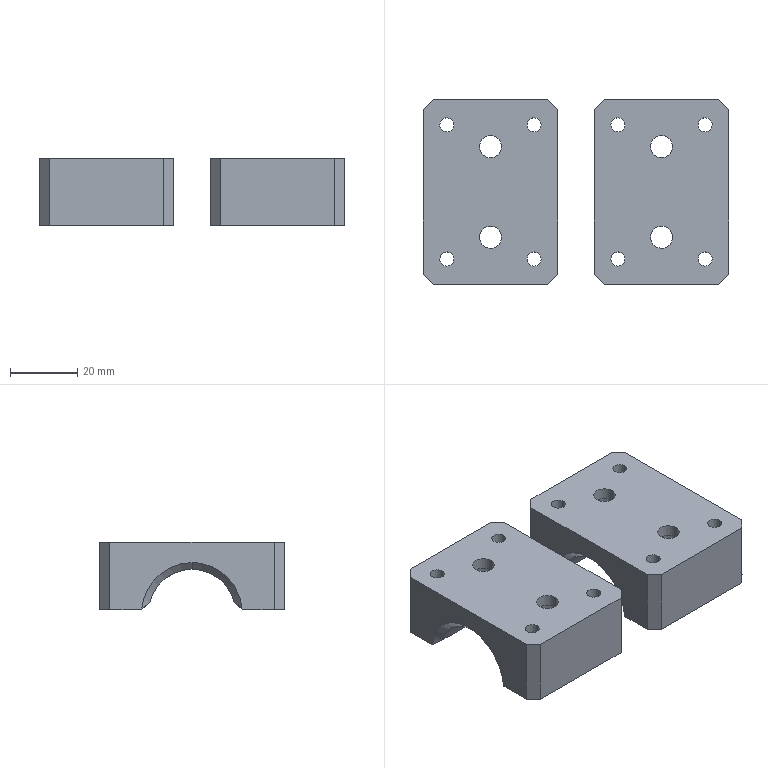Part | 2 solids | 76 faces | box 91 x 55 x 20 mm | volume 59531 mm3 | cylinder 36 | plane 34 | cone 6 | commonest cylinder face diameters 4.2 x16 6.6 x8 11 x8 26 x4